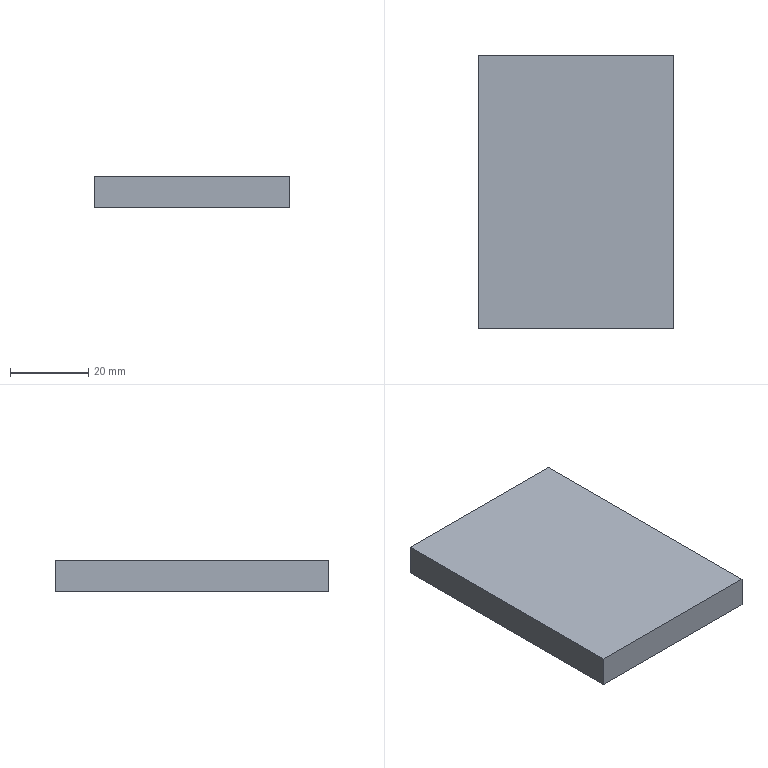Part | SolidWorks | features Extrusion 1 | 1 solid | 6 faces | box 50 x 70 x 8 mm | volume 28000 mm3 | plane 6
STEP:
#1=CARTESIAN_POINT('',(25.,-35.,-4.));
#2=VERTEX_POINT('',#1);
#3=CARTESIAN_POINT('',(25.,35.,-4.));
#4=VERTEX_POINT('',#3);
#5=CARTESIAN_POINT('',(25.,-35.,-4.));
#6=DIRECTION('',(0.,1.,0.));
#7=VECTOR('',#6,1000.);
#8=LINE('',#5,#7);
#9=EDGE_CURVE('',#2,#4,#8,.T.);
#10=ORIENTED_EDGE('',*,*,#9,.T.);
#11=CARTESIAN_POINT('',(25.,35.,4.));
#12=VERTEX_POINT('',#11);
#13=CARTESIAN_POINT('',(25.,35.,4.));
#14=DIRECTION('',(0.,0.,-1.));
#15=VECTOR('',#14,1000.);
#16=LINE('',#13,#15);
#17=EDGE_CURVE('',#12,#4,#16,.T.);
#18=ORIENTED_EDGE('',*,*,#17,.F.);
#19=CARTESIAN_POINT('',(25.,-35.,4.));
#20=VERTEX_POINT('',#19);
#21=CARTESIAN_POINT('',(25.,-35.,4.));
#22=DIRECTION('',(0.,1.,0.));
#23=VECTOR('',#22,1000.);
#24=LINE('',#21,#23);
#25=EDGE_CURVE('',#20,#12,#24,.T.);
#26=ORIENTED_EDGE('',*,*,#25,.F.);
#27=CARTESIAN_POINT('',(25.,-35.,4.));
#28=DIRECTION('',(0.,0.,-1.));
#29=VECTOR('',#28,1000.);
#30=LINE('',#27,#29);
#31=EDGE_CURVE('',#20,#2,#30,.T.);
#32=ORIENTED_EDGE('',*,*,#31,.T.);
#33=EDGE_LOOP('',(#10,#18,#26,#32));
#34=FACE_OUTER_BOUND('',#33,.T.);
#35=CARTESIAN_POINT('',(25.,-35.,4.));
#36=DIRECTION('',(-1.,0.,0.));
#37=DIRECTION('',(0.,0.,1.));
#38=AXIS2_PLACEMENT_3D('',#35,#36,#37);
#39=PLANE('',#38);
#40=ADVANCED_FACE('',(#34),#39,.F.);
#41=CARTESIAN_POINT('',(-25.,35.,-4.));
#42=VERTEX_POINT('',#41);
#43=CARTESIAN_POINT('',(-25.,35.,-4.));
#44=DIRECTION('',(-1.,0.,0.));
#45=VECTOR('',#44,1000.);
#46=LINE('',#43,#45);
#47=EDGE_CURVE('',#4,#42,#46,.T.);
#48=ORIENTED_EDGE('',*,*,#47,.T.);
#49=CARTESIAN_POINT('',(-25.,35.,4.));
#50=VERTEX_POINT('',#49);
#51=CARTESIAN_POINT('',(-25.,35.,4.));
#52=DIRECTION('',(0.,0.,-1.));
#53=VECTOR('',#52,1000.);
#54=LINE('',#51,#53);
#55=EDGE_CURVE('',#50,#42,#54,.T.);
#56=ORIENTED_EDGE('',*,*,#55,.F.);
#57=CARTESIAN_POINT('',(-25.,35.,4.));
#58=DIRECTION('',(-1.,0.,0.));
#59=VECTOR('',#58,1000.);
#60=LINE('',#57,#59);
#61=EDGE_CURVE('',#12,#50,#60,.T.);
#62=ORIENTED_EDGE('',*,*,#61,.F.);
#63=ORIENTED_EDGE('',*,*,#17,.T.);
#64=EDGE_LOOP('',(#48,#56,#62,#63));
#65=FACE_OUTER_BOUND('',#64,.T.);
#66=CARTESIAN_POINT('',(-25.,35.,4.));
#67=DIRECTION('',(0.,-1.,0.));
#68=DIRECTION('',(0.,0.,-1.));
#69=AXIS2_PLACEMENT_3D('',#66,#67,#68);
#70=PLANE('',#69);
#71=ADVANCED_FACE('',(#65),#70,.F.);
#72=CARTESIAN_POINT('',(-25.,-35.,-4.));
#73=VERTEX_POINT('',#72);
#74=CARTESIAN_POINT('',(-25.,-35.,-4.));
#75=DIRECTION('',(0.,-1.,0.));
#76=VECTOR('',#75,1000.);
#77=LINE('',#74,#76);
#78=EDGE_CURVE('',#42,#73,#77,.T.);
#79=ORIENTED_EDGE('',*,*,#78,.T.);
#80=CARTESIAN_POINT('',(-25.,-35.,4.));
#81=VERTEX_POINT('',#80);
#82=CARTESIAN_POINT('',(-25.,-35.,4.));
#83=DIRECTION('',(0.,0.,-1.));
#84=VECTOR('',#83,1000.);
#85=LINE('',#82,#84);
#86=EDGE_CURVE('',#81,#73,#85,.T.);
#87=ORIENTED_EDGE('',*,*,#86,.F.);
#88=CARTESIAN_POINT('',(-25.,-35.,4.));
#89=DIRECTION('',(0.,-1.,0.));
#90=VECTOR('',#89,1000.);
#91=LINE('',#88,#90);
#92=EDGE_CURVE('',#50,#81,#91,.T.);
#93=ORIENTED_EDGE('',*,*,#92,.F.);
#94=ORIENTED_EDGE('',*,*,#55,.T.);
#95=EDGE_LOOP('',(#79,#87,#93,#94));
#96=FACE_OUTER_BOUND('',#95,.T.);
#97=CARTESIAN_POINT('',(-25.,-35.,4.));
#98=DIRECTION('',(1.,0.,0.));
#99=DIRECTION('',(0.,0.,-1.));
#100=AXIS2_PLACEMENT_3D('',#97,#98,#99);
#101=PLANE('',#100);
#102=ADVANCED_FACE('',(#96),#101,.F.);
#103=CARTESIAN_POINT('',(-25.,-35.,-4.));
#104=DIRECTION('',(1.,0.,0.));
#105=VECTOR('',#104,1000.);
#106=LINE('',#103,#105);
#107=EDGE_CURVE('',#73,#2,#106,.T.);
#108=ORIENTED_EDGE('',*,*,#107,.T.);
#109=ORIENTED_EDGE('',*,*,#31,.F.);
#110=CARTESIAN_POINT('',(-25.,-35.,4.));
#111=DIRECTION('',(1.,0.,0.));
#112=VECTOR('',#111,1000.);
#113=LINE('',#110,#112);
#114=EDGE_CURVE('',#81,#20,#113,.T.);
#115=ORIENTED_EDGE('',*,*,#114,.F.);
#116=ORIENTED_EDGE('',*,*,#86,.T.);
#117=EDGE_LOOP('',(#108,#109,#115,#116));
#118=FACE_OUTER_BOUND('',#117,.T.);
#119=CARTESIAN_POINT('',(-25.,-35.,4.));
#120=DIRECTION('',(0.,1.,0.));
#121=DIRECTION('',(0.,0.,1.));
#122=AXIS2_PLACEMENT_3D('',#119,#120,#121);
#123=PLANE('',#122);
#124=ADVANCED_FACE('',(#118),#123,.F.);
#125=ORIENTED_EDGE('',*,*,#25,.T.);
#126=ORIENTED_EDGE('',*,*,#61,.T.);
#127=ORIENTED_EDGE('',*,*,#92,.T.);
#128=ORIENTED_EDGE('',*,*,#114,.T.);
#129=EDGE_LOOP('',(#125,#126,#127,#128));
#130=FACE_OUTER_BOUND('',#129,.T.);
#131=CARTESIAN_POINT('',(0.,0.,4.));
#132=DIRECTION('',(0.,0.,-1.));
#133=DIRECTION('',(-1.,0.,0.));
#134=AXIS2_PLACEMENT_3D('',#131,#132,#133);
#135=PLANE('',#134);
#136=ADVANCED_FACE('',(#130),#135,.F.);
#137=ORIENTED_EDGE('',*,*,#9,.F.);
#138=ORIENTED_EDGE('',*,*,#107,.F.);
#139=ORIENTED_EDGE('',*,*,#78,.F.);
#140=ORIENTED_EDGE('',*,*,#47,.F.);
#141=EDGE_LOOP('',(#137,#138,#139,#140));
#142=FACE_OUTER_BOUND('',#141,.T.);
#143=CARTESIAN_POINT('',(0.,0.,-4.));
#144=DIRECTION('',(0.,0.,-1.));
#145=DIRECTION('',(-1.,0.,0.));
#146=AXIS2_PLACEMENT_3D('',#143,#144,#145);
#147=PLANE('',#146);
#148=ADVANCED_FACE('',(#142),#147,.T.);
#149=CLOSED_SHELL('',(#40,#71,#102,#124,#136,#148));
#150=MANIFOLD_SOLID_BREP('',#149);
#151=CARTESIAN_POINT('',(0.,0.,0.));
#152=DIRECTION('',(0.,0.,1.));
#153=DIRECTION('',(1.,0.,0.));
#154=AXIS2_PLACEMENT_3D('',#151,#152,#153);
#155=(LENGTH_UNIT()NAMED_UNIT(*)SI_UNIT(.MILLI.,.METRE.));
#156=UNCERTAINTY_MEASURE_WITH_UNIT(LENGTH_MEASURE(0.00001),#155,'','');
#157=(NAMED_UNIT(*)PLANE_ANGLE_UNIT()SI_UNIT($,.RADIAN.));
#158=(NAMED_UNIT(*)SI_UNIT($,.STERADIAN.)SOLID_ANGLE_UNIT());
#159=(GEOMETRIC_REPRESENTATION_CONTEXT(3)GLOBAL_UNCERTAINTY_ASSIGNED_CONTEXT((#156))GLOBAL_UNIT_ASSIGNED_CONTEXT((#155,#157,#158))REPRESENTATION_CONTEXT('',''));
#160=ADVANCED_BREP_SHAPE_REPRESENTATION('',(#150,#154),#159);